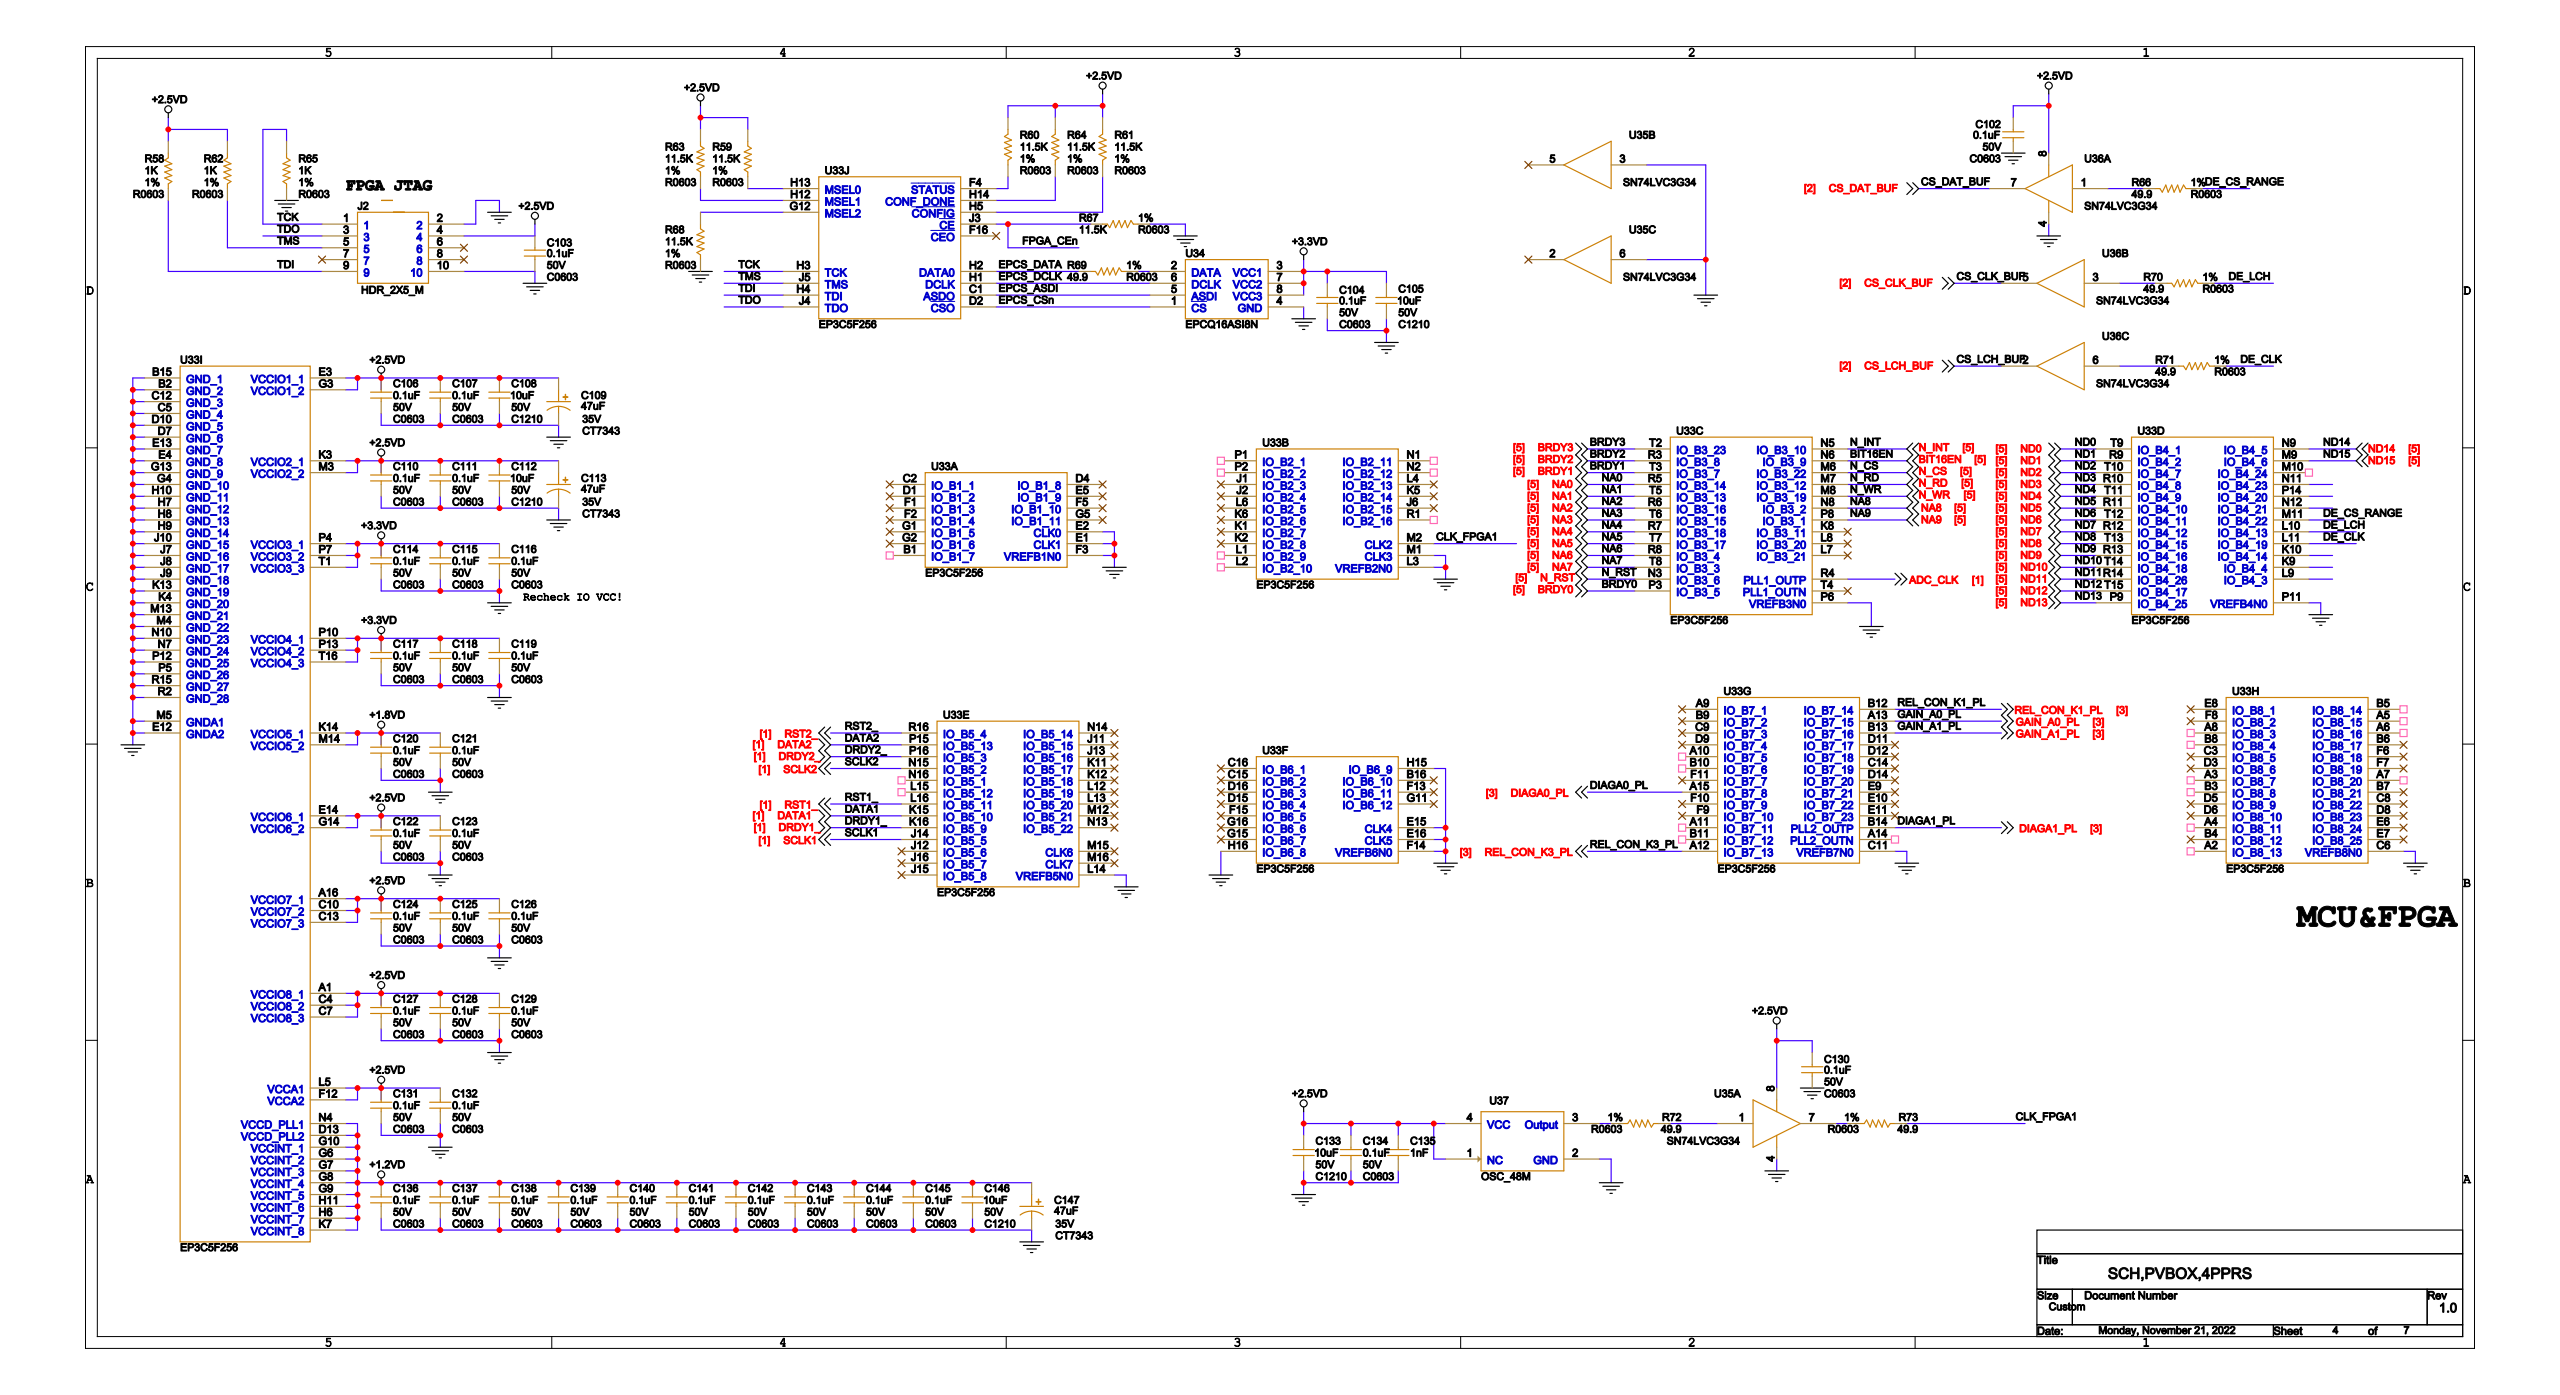Circuit board | Cadence Allegro | 405 parts | 254 nets | one sheet of the schematic
Parts on this sheet (reference | value | footprint):
C102 | C0603
C103 | C0603
C104 | C0603
C105 | C1210
C106 | C0603
C107 | C0603
C108 | C1210
C109 | CT7343
C110 | C0603
C111 | C0603
C112 | C1210
C113 | CT7343
C114 | C0603
C115 | C0603
C116 | C0603
C117 | C0603
C118 | C0603
C119 | C0603
C120 | C0603
C121 | C0603
C122 | C0603
C123 | C0603
C124 | C0603
C125 | C0603
C126 | C0603
C127 | C0603
C128 | C0603
C129 | C0603
C130 | C0603
C131 | C0603
C132 | C0603
C133 | C1210
C134 | C0603
C135 | C0603
C136 | C0603
C137 | C0603
C138 | C0603
C139 | C0603
C140 | C0603
C141 | C0603
C142 | C0603
C143 | C0603
C144 | C0603
C145 | C0603
C146 | C1210
C147 | CT7343
J2 | N2510_6002RB
R4 | R0603
R58 | R0603
R59 | R0603
R60 | R0603
R61 | R0603
R62 | R0603
R63 | R0603
R64 | R0603
R65 | R0603
R66 | R0603
R67 | R0603
R68 | R0603
R69 | R0603
R70 | R0603
R71 | R0603
R72 | R0603
R73 | R0603
U33 | BGA_256_17MX17MX1M55_1M
U34 | SOIC_8_4MX5MX1M75_1M27
U37 | CO4-5R0X7R0-S
Nets of these parts (net: part-pin ...):
GND: C102-2 C103-2 C104-2 C105-2 C106-2 C107-2 C108-2 C109-2 C110-2 C111-2 C112-2 C113-2 C114-2 C115-2 C116-2 C117-2 C118-2 C119-2 C120-2 C121-2 C122-2 C123-2 C124-2 C125-2 C126-2 C127-2 C128-2 C129-2 C130-2 C131-2 C132-2 C133-2 C134-2 C135-2 C136-2 C137-2 C138-2 C139-2 C140-2 C141-2 C142-2 C143-2 C144-2 C145-2 C146-2 C147-2 J2-2 J2-10 R4-1 R65-1 R67-2 R68-2 U34-4 U37-2 U33-B2 U33-B15 U33-C5 U33-C6 U33-C11 U33-C12 U33-D7 U33-D10 U33-E1 U33-E2 U33-E4 U33-E12 U33-E13 U33-E15 U33-E16 U33-F3 U33-F14 U33-G4 U33-G13 U33-H7 U33-H8 U33-H9 U33-H10 U33-H15 U33-H16 U33-J7 U33-J8 U33-J9 U33-J10 U33-K4 U33-K13 U33-L3 U33-L14 U33-M1 U33-M4 U33-M5 U33-M13 U33-N7 U33-N10 U33-P5 U33-P6 U33-P11 U33-P12 U33-R2 U33-R15
N19763949: R66-1
DE_CS_RANGE: R66-2 U33-M11
EPCS_DATA: R69-1 U33-H2
N19337370: R69-2 U34-2
ADC_CLK: U33-R4
N19765979: R70-1
DE_LCH: R70-2 U33-L10
N19765974: R71-1
DE_CLK: R71-2 U33-L11
N17410279: R72-1
N19358042: R72-2 U37-3
CLK_FPGA1: R73-1 U33-M2
N17410283: R73-2
N16962547: R4-2
+2.5VD: C102-1 C103-1 C106-1 C107-1 C108-1 C109-1 C110-1 C111-1 C112-1 C113-1 C122-1 C123-1 C124-1 C125-1 C126-1 C127-1 C128-1 C129-1 C130-1 C131-1 C132-1 C133-1 C134-1 C135-1 J2-4 R58-2 R59-1 R60-1 R61-1 R62-2 R63-1 R64-1 U37-1 U37-4 U33-A1 U33-A16 U33-C4 U33-C7 U33-C10 U33-C13 U33-E3 U33-E14 U33-F12 U33-G3 U33-G14 U33-K3 U33-L5 U33-M3
+3.3VD: C104-1 C105-1 C114-1 C115-1 C116-1 C117-1 C118-1 C119-1 U34-3 U34-7 U34-8 U33-P4 U33-P7 U33-P10 U33-P13 U33-T1 U33-T16
+1.8VD: C120-1 C121-1 U33-K14 U33-M14
+1.2VD: C136-1 C137-1 C138-1 C139-1 C140-1 C141-1 C142-1 C143-1 C144-1 C145-1 C146-1 C147-1 U33-D13 U33-G6 U33-G7 U33-G8 U33-G9 U33-G10 U33-H6 U33-H11 U33-K7 U33-N4
TCK: J2-1 R65-2 U33-H3
TDO: J2-3 U33-J4
TMS: J2-5 R62-1 U33-J5
TDI: J2-9 R58-1 U33-H4
N19337262: R59-2 U33-H13
N19337254: R60-2 U33-F4
N19337258: R61-2 U33-H5
N19337260: R63-2 U33-H12
N19337256: R64-2 U33-H14
FPGA_CEN: R67-1 U33-J3
N19337284: R68-1 U33-G12
REL_CON_K3_PL: U33-A12
REL_CON_K1_PL: U33-B12
GAIN_A0_PL: U33-A13
GAIN_A1_PL: U33-B13
DIAGA1_PL: U33-B14
DIAGA0_PL: U33-A15
DATA1: U33-K15
DRDY1_: U33-K16
SCLK1: U33-J14
RST1_: U33-L16
DATA2: U33-P15
DRDY2_: U33-P16
SCLK2: U33-N15
RST2_: U33-R16
NA9: U33-P8
N_INT: U33-N5
N_RD: U33-M7
NA1: U33-T5
NA0: U33-R5
NA3: U33-T6
NA2: U33-R6
NA5: U33-T7
NA4: U33-R7
N_WR: U33-M8
NA8: U33-N8
N_CS: U33-M6
BRDY3: U33-T2
NA7: U33-T8
NA6: U33-R8
BRDY0: U33-P3
N_RST: U33-N3
BRDY1: U33-T3
BRDY2: U33-R3
BIT16EN: U33-N6
ND0: U33-T9
ND5: U33-R11
ND6: U33-T12
ND7: U33-R12
ND8: U33-T13
ND9: U33-R13
ND12: U33-T15
ND10: U33-T14
ND1: U33-R9
ND13: U33-P9
ND11: U33-R14
ND14: U33-N9
ND15: U33-M9
ND2: U33-T10
ND3: U33-R10
ND4: U33-T11
EPCS_ASDI: U34-5 U33-C1
EPCS_CSN: U34-1 U33-D2
EPCS_DCLK: U34-6 U33-H1